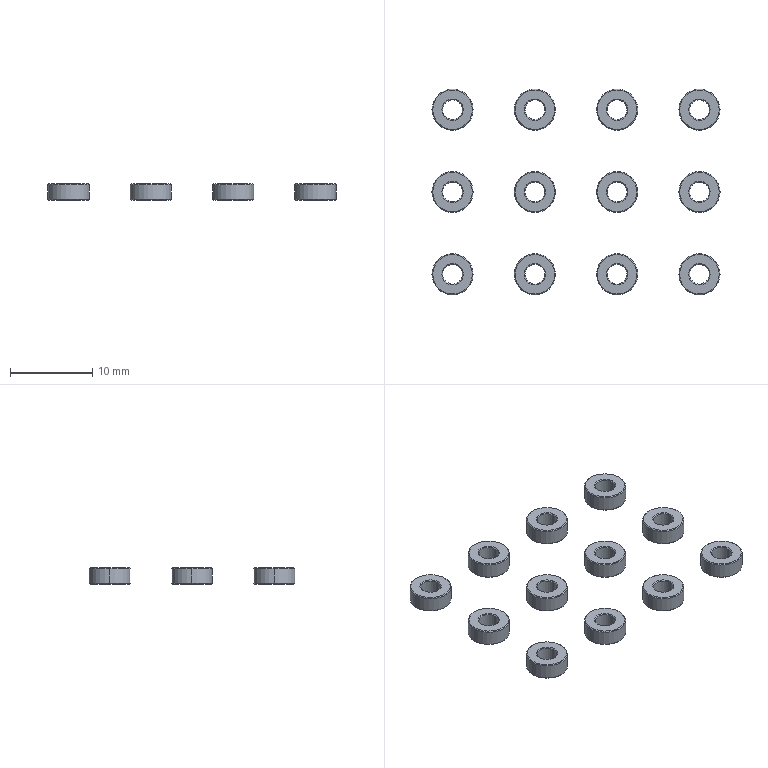Part | 12 solids | 168 faces | box 35 x 25 x 2 mm | volume 359.876 mm3 | cone 96 | cylinder 48 | plane 24 | commonest cylinder face diameters 2.4 x24 5 x24